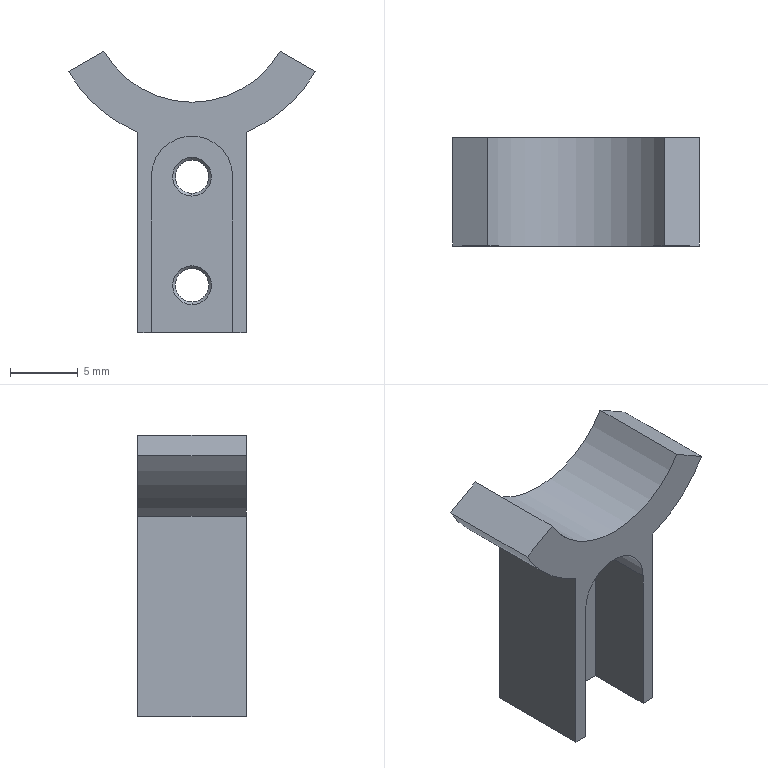Part | STEP file | jaw_5 | 1 solid | 27 faces | box 18.187 x 8 x 20.75 mm | volume 920.185 mm3 | plane 10 | cone 9 | cylinder 8 | commonest cylinder face diameters 2.459 x4 21 x2 6 x1 15 x1